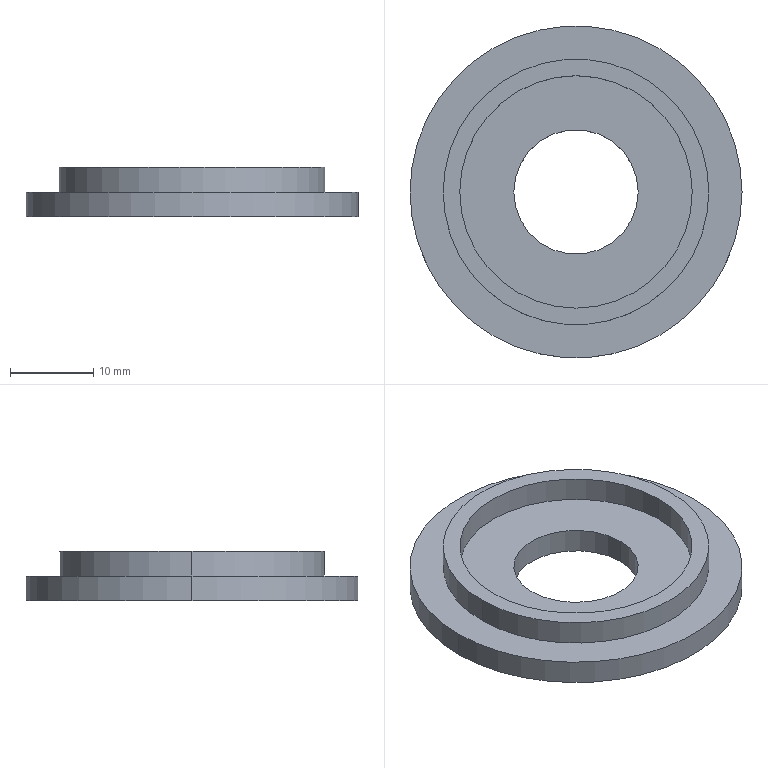Part | STEP file | inner seal | 1 solid | 12 faces | box 40 x 40 x 6 mm | volume 3805 mm3 | cylinder 8 | plane 4 | commonest cylinder face diameters 15 x2 28 x2 32 x2 40 x2
STEP:
#1=CARTESIAN_POINT('',(-7.5,0.,0.));
#2=VERTEX_POINT('',#1);
#3=CARTESIAN_POINT('',(7.5,0.,0.));
#4=VERTEX_POINT('',#3);
#5=CARTESIAN_POINT('',(0.,0.,0.));
#6=DIRECTION('',(0.,0.,1.));
#7=DIRECTION('',(1.,0.,0.));
#8=AXIS2_PLACEMENT_3D('',#5,#6,#7);
#9=CIRCLE('',#8,7.5);
#10=EDGE_CURVE('',#2,#4,#9,.T.);
#11=ORIENTED_EDGE('',*,*,#10,.F.);
#12=CARTESIAN_POINT('',(-7.5,0.,3.));
#13=VERTEX_POINT('',#12);
#14=CARTESIAN_POINT('',(-7.5,0.,0.));
#15=DIRECTION('',(0.,0.,1.));
#16=VECTOR('',#15,1000.);
#17=LINE('',#14,#16);
#18=EDGE_CURVE('',#2,#13,#17,.T.);
#19=ORIENTED_EDGE('',*,*,#18,.T.);
#20=CARTESIAN_POINT('',(7.5,0.,3.));
#21=VERTEX_POINT('',#20);
#22=CARTESIAN_POINT('',(0.,0.,3.));
#23=DIRECTION('',(0.,0.,1.));
#24=DIRECTION('',(1.,0.,0.));
#25=AXIS2_PLACEMENT_3D('',#22,#23,#24);
#26=CIRCLE('',#25,7.5);
#27=EDGE_CURVE('',#13,#21,#26,.T.);
#28=ORIENTED_EDGE('',*,*,#27,.T.);
#29=CARTESIAN_POINT('',(7.5,0.,0.));
#30=DIRECTION('',(0.,0.,1.));
#31=VECTOR('',#30,1000.);
#32=LINE('',#29,#31);
#33=EDGE_CURVE('',#4,#21,#32,.T.);
#34=ORIENTED_EDGE('',*,*,#33,.F.);
#35=EDGE_LOOP('',(#11,#19,#28,#34));
#36=FACE_OUTER_BOUND('',#35,.T.);
#37=CARTESIAN_POINT('',(0.,0.,0.));
#38=DIRECTION('',(0.,0.,1.));
#39=DIRECTION('',(1.,0.,0.));
#40=AXIS2_PLACEMENT_3D('',#37,#38,#39);
#41=CYLINDRICAL_SURFACE('',#40,7.5);
#42=ADVANCED_FACE('',(#36),#41,.F.);
#43=CARTESIAN_POINT('',(-14.,0.,6.));
#44=VERTEX_POINT('',#43);
#45=CARTESIAN_POINT('',(14.,0.,6.));
#46=VERTEX_POINT('',#45);
#47=CARTESIAN_POINT('',(0.,0.,6.));
#48=DIRECTION('',(0.,0.,1.));
#49=DIRECTION('',(1.,0.,0.));
#50=AXIS2_PLACEMENT_3D('',#47,#48,#49);
#51=CIRCLE('',#50,14.);
#52=EDGE_CURVE('',#44,#46,#51,.T.);
#53=ORIENTED_EDGE('',*,*,#52,.T.);
#54=CARTESIAN_POINT('',(14.,0.,3.));
#55=VERTEX_POINT('',#54);
#56=CARTESIAN_POINT('',(14.,0.,6.));
#57=DIRECTION('',(0.,0.,-1.));
#58=VECTOR('',#57,1000.);
#59=LINE('',#56,#58);
#60=EDGE_CURVE('',#46,#55,#59,.T.);
#61=ORIENTED_EDGE('',*,*,#60,.T.);
#62=CARTESIAN_POINT('',(-14.,0.,3.));
#63=VERTEX_POINT('',#62);
#64=CARTESIAN_POINT('',(0.,0.,3.));
#65=DIRECTION('',(0.,0.,-1.));
#66=DIRECTION('',(1.,0.,0.));
#67=AXIS2_PLACEMENT_3D('',#64,#65,#66);
#68=CIRCLE('',#67,14.);
#69=EDGE_CURVE('',#55,#63,#68,.T.);
#70=ORIENTED_EDGE('',*,*,#69,.T.);
#71=CARTESIAN_POINT('',(-14.,0.,6.));
#72=DIRECTION('',(0.,0.,-1.));
#73=VECTOR('',#72,1000.);
#74=LINE('',#71,#73);
#75=EDGE_CURVE('',#44,#63,#74,.T.);
#76=ORIENTED_EDGE('',*,*,#75,.F.);
#77=EDGE_LOOP('',(#53,#61,#70,#76));
#78=FACE_OUTER_BOUND('',#77,.T.);
#79=CARTESIAN_POINT('',(0.,0.,6.));
#80=DIRECTION('',(0.,0.,-1.));
#81=DIRECTION('',(-1.,0.,0.));
#82=AXIS2_PLACEMENT_3D('',#79,#80,#81);
#83=CYLINDRICAL_SURFACE('',#82,14.);
#84=ADVANCED_FACE('',(#78),#83,.F.);
#85=CARTESIAN_POINT('',(16.,0.,6.));
#86=VERTEX_POINT('',#85);
#87=CARTESIAN_POINT('',(-16.,0.,6.));
#88=VERTEX_POINT('',#87);
#89=CARTESIAN_POINT('',(0.,0.,6.));
#90=DIRECTION('',(0.,0.,1.));
#91=DIRECTION('',(1.,0.,0.));
#92=AXIS2_PLACEMENT_3D('',#89,#90,#91);
#93=CIRCLE('',#92,16.);
#94=EDGE_CURVE('',#86,#88,#93,.T.);
#95=ORIENTED_EDGE('',*,*,#94,.F.);
#96=CARTESIAN_POINT('',(16.,0.,3.));
#97=VERTEX_POINT('',#96);
#98=CARTESIAN_POINT('',(16.,0.,6.));
#99=DIRECTION('',(0.,0.,-1.));
#100=VECTOR('',#99,1000.);
#101=LINE('',#98,#100);
#102=EDGE_CURVE('',#86,#97,#101,.T.);
#103=ORIENTED_EDGE('',*,*,#102,.T.);
#104=CARTESIAN_POINT('',(-16.,0.,3.));
#105=VERTEX_POINT('',#104);
#106=CARTESIAN_POINT('',(0.,0.,3.));
#107=DIRECTION('',(0.,0.,1.));
#108=DIRECTION('',(1.,0.,0.));
#109=AXIS2_PLACEMENT_3D('',#106,#107,#108);
#110=CIRCLE('',#109,16.);
#111=EDGE_CURVE('',#97,#105,#110,.T.);
#112=ORIENTED_EDGE('',*,*,#111,.T.);
#113=CARTESIAN_POINT('',(-16.,0.,6.));
#114=DIRECTION('',(0.,0.,-1.));
#115=VECTOR('',#114,1000.);
#116=LINE('',#113,#115);
#117=EDGE_CURVE('',#88,#105,#116,.T.);
#118=ORIENTED_EDGE('',*,*,#117,.F.);
#119=EDGE_LOOP('',(#95,#103,#112,#118));
#120=FACE_OUTER_BOUND('',#119,.T.);
#121=CARTESIAN_POINT('',(0.,0.,6.));
#122=DIRECTION('',(0.,0.,-1.));
#123=DIRECTION('',(-1.,0.,0.));
#124=AXIS2_PLACEMENT_3D('',#121,#122,#123);
#125=CYLINDRICAL_SURFACE('',#124,16.);
#126=ADVANCED_FACE('',(#120),#125,.T.);
#127=CARTESIAN_POINT('',(20.,0.,3.));
#128=VERTEX_POINT('',#127);
#129=CARTESIAN_POINT('',(-20.,0.,3.));
#130=VERTEX_POINT('',#129);
#131=CARTESIAN_POINT('',(0.,0.,3.));
#132=DIRECTION('',(0.,0.,1.));
#133=DIRECTION('',(1.,0.,0.));
#134=AXIS2_PLACEMENT_3D('',#131,#132,#133);
#135=CIRCLE('',#134,20.);
#136=EDGE_CURVE('',#128,#130,#135,.T.);
#137=ORIENTED_EDGE('',*,*,#136,.F.);
#138=CARTESIAN_POINT('',(20.,0.,0.));
#139=VERTEX_POINT('',#138);
#140=CARTESIAN_POINT('',(20.,0.,3.));
#141=DIRECTION('',(0.,0.,-1.));
#142=VECTOR('',#141,1000.);
#143=LINE('',#140,#142);
#144=EDGE_CURVE('',#128,#139,#143,.T.);
#145=ORIENTED_EDGE('',*,*,#144,.T.);
#146=CARTESIAN_POINT('',(-20.,0.,0.));
#147=VERTEX_POINT('',#146);
#148=CARTESIAN_POINT('',(0.,0.,0.));
#149=DIRECTION('',(0.,0.,1.));
#150=DIRECTION('',(1.,0.,0.));
#151=AXIS2_PLACEMENT_3D('',#148,#149,#150);
#152=CIRCLE('',#151,20.);
#153=EDGE_CURVE('',#139,#147,#152,.T.);
#154=ORIENTED_EDGE('',*,*,#153,.T.);
#155=CARTESIAN_POINT('',(-20.,0.,3.));
#156=DIRECTION('',(0.,0.,-1.));
#157=VECTOR('',#156,1000.);
#158=LINE('',#155,#157);
#159=EDGE_CURVE('',#130,#147,#158,.T.);
#160=ORIENTED_EDGE('',*,*,#159,.F.);
#161=EDGE_LOOP('',(#137,#145,#154,#160));
#162=FACE_OUTER_BOUND('',#161,.T.);
#163=CARTESIAN_POINT('',(0.,0.,3.));
#164=DIRECTION('',(0.,0.,-1.));
#165=DIRECTION('',(-1.,0.,0.));
#166=AXIS2_PLACEMENT_3D('',#163,#164,#165);
#167=CYLINDRICAL_SURFACE('',#166,20.);
#168=ADVANCED_FACE('',(#162),#167,.T.);
#169=ORIENTED_EDGE('',*,*,#144,.F.);
#170=CARTESIAN_POINT('',(0.,0.,3.));
#171=DIRECTION('',(0.,0.,1.));
#172=DIRECTION('',(1.,0.,0.));
#173=AXIS2_PLACEMENT_3D('',#170,#171,#172);
#174=CIRCLE('',#173,20.);
#175=EDGE_CURVE('',#130,#128,#174,.T.);
#176=ORIENTED_EDGE('',*,*,#175,.F.);
#177=ORIENTED_EDGE('',*,*,#159,.T.);
#178=CARTESIAN_POINT('',(0.,0.,0.));
#179=DIRECTION('',(0.,0.,1.));
#180=DIRECTION('',(1.,0.,0.));
#181=AXIS2_PLACEMENT_3D('',#178,#179,#180);
#182=CIRCLE('',#181,20.);
#183=EDGE_CURVE('',#147,#139,#182,.T.);
#184=ORIENTED_EDGE('',*,*,#183,.T.);
#185=EDGE_LOOP('',(#169,#176,#177,#184));
#186=FACE_OUTER_BOUND('',#185,.T.);
#187=CARTESIAN_POINT('',(0.,0.,3.));
#188=DIRECTION('',(0.,0.,-1.));
#189=DIRECTION('',(-1.,0.,0.));
#190=AXIS2_PLACEMENT_3D('',#187,#188,#189);
#191=CYLINDRICAL_SURFACE('',#190,20.);
#192=ADVANCED_FACE('',(#186),#191,.T.);
#193=CARTESIAN_POINT('',(0.,0.,3.));
#194=DIRECTION('',(0.,0.,1.));
#195=DIRECTION('',(1.,0.,0.));
#196=AXIS2_PLACEMENT_3D('',#193,#194,#195);
#197=CIRCLE('',#196,16.);
#198=EDGE_CURVE('',#105,#97,#197,.T.);
#199=ORIENTED_EDGE('',*,*,#198,.F.);
#200=ORIENTED_EDGE('',*,*,#111,.F.);
#201=EDGE_LOOP('',(#199,#200));
#202=FACE_BOUND('',#201,.T.);
#203=ORIENTED_EDGE('',*,*,#175,.T.);
#204=ORIENTED_EDGE('',*,*,#136,.T.);
#205=EDGE_LOOP('',(#203,#204));
#206=FACE_OUTER_BOUND('',#205,.T.);
#207=CARTESIAN_POINT('',(0.,0.,3.));
#208=DIRECTION('',(0.,0.,1.));
#209=DIRECTION('',(1.,0.,0.));
#210=AXIS2_PLACEMENT_3D('',#207,#208,#209);
#211=PLANE('',#210);
#212=ADVANCED_FACE('',(#202,#206),#211,.T.);
#213=CARTESIAN_POINT('',(0.,0.,0.));
#214=DIRECTION('',(0.,0.,1.));
#215=DIRECTION('',(1.,0.,0.));
#216=AXIS2_PLACEMENT_3D('',#213,#214,#215);
#217=CIRCLE('',#216,7.5);
#218=EDGE_CURVE('',#4,#2,#217,.T.);
#219=ORIENTED_EDGE('',*,*,#218,.T.);
#220=ORIENTED_EDGE('',*,*,#10,.T.);
#221=EDGE_LOOP('',(#219,#220));
#222=FACE_BOUND('',#221,.T.);
#223=ORIENTED_EDGE('',*,*,#183,.F.);
#224=ORIENTED_EDGE('',*,*,#153,.F.);
#225=EDGE_LOOP('',(#223,#224));
#226=FACE_OUTER_BOUND('',#225,.T.);
#227=CARTESIAN_POINT('',(0.,0.,0.));
#228=DIRECTION('',(0.,0.,1.));
#229=DIRECTION('',(1.,0.,0.));
#230=AXIS2_PLACEMENT_3D('',#227,#228,#229);
#231=PLANE('',#230);
#232=ADVANCED_FACE('',(#222,#226),#231,.F.);
#233=CARTESIAN_POINT('',(0.,0.,6.));
#234=DIRECTION('',(0.,0.,1.));
#235=DIRECTION('',(1.,0.,0.));
#236=AXIS2_PLACEMENT_3D('',#233,#234,#235);
#237=CIRCLE('',#236,16.);
#238=EDGE_CURVE('',#88,#86,#237,.T.);
#239=ORIENTED_EDGE('',*,*,#238,.T.);
#240=ORIENTED_EDGE('',*,*,#94,.T.);
#241=EDGE_LOOP('',(#239,#240));
#242=FACE_OUTER_BOUND('',#241,.T.);
#243=ORIENTED_EDGE('',*,*,#52,.F.);
#244=CARTESIAN_POINT('',(0.,0.,6.));
#245=DIRECTION('',(0.,0.,1.));
#246=DIRECTION('',(1.,0.,0.));
#247=AXIS2_PLACEMENT_3D('',#244,#245,#246);
#248=CIRCLE('',#247,14.);
#249=EDGE_CURVE('',#46,#44,#248,.T.);
#250=ORIENTED_EDGE('',*,*,#249,.F.);
#251=EDGE_LOOP('',(#243,#250));
#252=FACE_BOUND('',#251,.T.);
#253=CARTESIAN_POINT('',(0.,0.,6.));
#254=DIRECTION('',(0.,0.,1.));
#255=DIRECTION('',(1.,0.,0.));
#256=AXIS2_PLACEMENT_3D('',#253,#254,#255);
#257=PLANE('',#256);
#258=ADVANCED_FACE('',(#242,#252),#257,.T.);
#259=ORIENTED_EDGE('',*,*,#102,.F.);
#260=ORIENTED_EDGE('',*,*,#238,.F.);
#261=ORIENTED_EDGE('',*,*,#117,.T.);
#262=ORIENTED_EDGE('',*,*,#198,.T.);
#263=EDGE_LOOP('',(#259,#260,#261,#262));
#264=FACE_OUTER_BOUND('',#263,.T.);
#265=CARTESIAN_POINT('',(0.,0.,6.));
#266=DIRECTION('',(0.,0.,-1.));
#267=DIRECTION('',(-1.,0.,0.));
#268=AXIS2_PLACEMENT_3D('',#265,#266,#267);
#269=CYLINDRICAL_SURFACE('',#268,16.);
#270=ADVANCED_FACE('',(#264),#269,.T.);
#271=ORIENTED_EDGE('',*,*,#60,.F.);
#272=ORIENTED_EDGE('',*,*,#249,.T.);
#273=ORIENTED_EDGE('',*,*,#75,.T.);
#274=CARTESIAN_POINT('',(0.,0.,3.));
#275=DIRECTION('',(0.,0.,-1.));
#276=DIRECTION('',(1.,0.,0.));
#277=AXIS2_PLACEMENT_3D('',#274,#275,#276);
#278=CIRCLE('',#277,14.);
#279=EDGE_CURVE('',#63,#55,#278,.T.);
#280=ORIENTED_EDGE('',*,*,#279,.T.);
#281=EDGE_LOOP('',(#271,#272,#273,#280));
#282=FACE_OUTER_BOUND('',#281,.T.);
#283=CARTESIAN_POINT('',(0.,0.,6.));
#284=DIRECTION('',(0.,0.,-1.));
#285=DIRECTION('',(-1.,0.,0.));
#286=AXIS2_PLACEMENT_3D('',#283,#284,#285);
#287=CYLINDRICAL_SURFACE('',#286,14.);
#288=ADVANCED_FACE('',(#282),#287,.F.);
#289=CARTESIAN_POINT('',(0.,0.,3.));
#290=DIRECTION('',(0.,0.,1.));
#291=DIRECTION('',(1.,0.,0.));
#292=AXIS2_PLACEMENT_3D('',#289,#290,#291);
#293=CIRCLE('',#292,7.5);
#294=EDGE_CURVE('',#21,#13,#293,.T.);
#295=ORIENTED_EDGE('',*,*,#294,.F.);
#296=ORIENTED_EDGE('',*,*,#27,.F.);
#297=EDGE_LOOP('',(#295,#296));
#298=FACE_BOUND('',#297,.T.);
#299=ORIENTED_EDGE('',*,*,#279,.F.);
#300=ORIENTED_EDGE('',*,*,#69,.F.);
#301=EDGE_LOOP('',(#299,#300));
#302=FACE_OUTER_BOUND('',#301,.T.);
#303=CARTESIAN_POINT('',(0.,0.,3.));
#304=DIRECTION('',(0.,0.,1.));
#305=DIRECTION('',(1.,0.,0.));
#306=AXIS2_PLACEMENT_3D('',#303,#304,#305);
#307=PLANE('',#306);
#308=ADVANCED_FACE('',(#298,#302),#307,.T.);
#309=ORIENTED_EDGE('',*,*,#18,.F.);
#310=ORIENTED_EDGE('',*,*,#218,.F.);
#311=ORIENTED_EDGE('',*,*,#33,.T.);
#312=ORIENTED_EDGE('',*,*,#294,.T.);
#313=EDGE_LOOP('',(#309,#310,#311,#312));
#314=FACE_OUTER_BOUND('',#313,.T.);
#315=CARTESIAN_POINT('',(0.,0.,0.));
#316=DIRECTION('',(0.,0.,1.));
#317=DIRECTION('',(1.,0.,0.));
#318=AXIS2_PLACEMENT_3D('',#315,#316,#317);
#319=CYLINDRICAL_SURFACE('',#318,7.5);
#320=ADVANCED_FACE('',(#314),#319,.F.);
#321=CLOSED_SHELL('',(#42,#84,#126,#168,#192,#212,#232,#258,#270,#288,#308,#320));
#322=MANIFOLD_SOLID_BREP('',#321);
#323=CARTESIAN_POINT('',(0.,0.,0.));
#324=DIRECTION('',(0.,0.,1.));
#325=DIRECTION('',(1.,0.,0.));
#326=AXIS2_PLACEMENT_3D('',#323,#324,#325);
#327=(LENGTH_UNIT()NAMED_UNIT(*)SI_UNIT(.MILLI.,.METRE.));
#328=UNCERTAINTY_MEASURE_WITH_UNIT(LENGTH_MEASURE(0.00001),#327,'','');
#329=(NAMED_UNIT(*)PLANE_ANGLE_UNIT()SI_UNIT($,.RADIAN.));
#330=(NAMED_UNIT(*)SI_UNIT($,.STERADIAN.)SOLID_ANGLE_UNIT());
#331=(GEOMETRIC_REPRESENTATION_CONTEXT(3)GLOBAL_UNCERTAINTY_ASSIGNED_CONTEXT((#328))GLOBAL_UNIT_ASSIGNED_CONTEXT((#327,#329,#330))REPRESENTATION_CONTEXT('',''));
#332=ADVANCED_BREP_SHAPE_REPRESENTATION('',(#322,#326),#331);